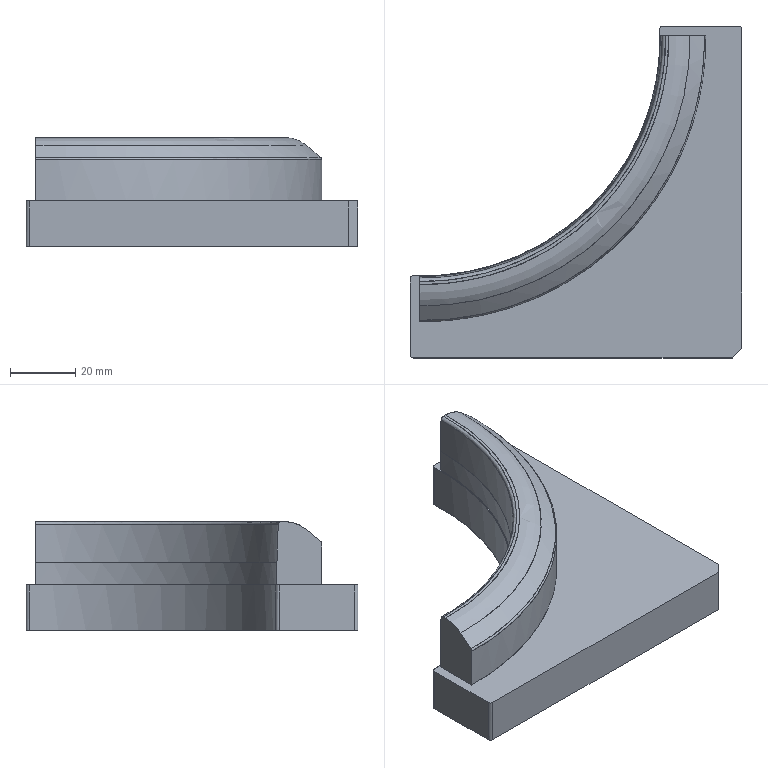NC program | PowerMill | posted with a generic post | part box 102 x 102 x 33.478 mm
Lines 26146 to 27280 of 205885:
N26243 M6
N26244 S8500 M03
N26245 G00 G90 X0.0 Y0.0
N26246 G43 Z11.798 H3
N26247
N26248 G05 P10000 R8
N26249 X37.5844 Y54.0857
N26250 Z0.7984
N26251 G01 Z-0.4016 F360.0
N26252 X33.1677 Y51.2016 F600.0
N26253 X22.0307 Y45.7859
N26254 X21.9859 Y44.2514
N26255 X21.9868 Y43.8083
N26256 X21.9186 Y42.9165
N26257 X21.8632 Y42.0238
N26258 X21.7548 Y40.6849
N26259 X21.6903 Y40.061
N26260 X34.2629 Y46.1749
N26261 X34.2244 Y44.6963
N26262 X34.2103 Y43.798
N26263 X34.1806 Y43.3523
N26264 X34.1258 Y42.0078
N26265 X33.9991 Y40.4872
N26266 X20.8197 Y34.0783
N26267 X20.719 Y33.5435
N26268 X20.4371 Y32.2041
N26269 X20.2385 Y31.3119
N26270 X19.7939 Y29.5261
N26271 X19.555 Y28.6339
N26272 X19.3094 Y27.7845
N26273 X33.3175 Y34.5964
N26274 X33.2791 Y34.4009
N26275 X33.2129 Y33.9562
N26276 X33.0631 Y33.0592
N26277 X32.8983 Y32.1648
N26278 X32.8079 Y31.717
N26279 X32.728 Y31.2672
N26280 X32.6288 Y30.8219
N26281 X32.4611 Y29.9296
N26282 X32.3634 Y29.4765
N26283 X32.2815 Y29.1526
N26284 X32.2658 Y29.0289
N26285 X32.1192 Y28.4543
N26286 X16.9967 Y21.1005
N26287 X16.8928 Y20.8373
N26288 X16.4531 Y19.7915
N26289 X16.0002 Y18.7513
N26290 X15.5539 Y17.7745
N26291 X15.1078 Y16.842
N26292 X14.3017 Y15.2433
N26293 X13.5777 Y13.8786
N26294 X30.3315 Y22.0256
N26295 X29.9768 Y20.977
N26296 X29.8344 Y20.5279
N26297 X29.5964 Y19.8574
N26298 X29.5319 Y19.6308
N26299 X29.3568 Y19.1846
N26300 X28.517 Y16.9457
N26301 X28.2532 Y16.3376
N26302 X28.1539 Y16.058
N26303 X27.799 Y15.2347
N26304 X8.4035 Y5.803
N26305 X7.438 Y4.5314
N26306 X6.6273 Y3.5171
N26307 X5.6141 Y2.2997
N26308 X4.4534 Y0.9605
N26309 X3.6379 Y0.0682
N26310 X2.3615 Y-1.271
N26311 X1.2711 Y-2.3584
N26312 X0.0766 Y-3.5028
N26313 X-0.6368 Y-4.1524
N26314 X24.2797 Y7.964
N26315 X23.6272 Y6.8079
N26316 X23.0209 Y5.7571
N26317 X22.8817 Y5.5385
N26318 X22.4904 Y4.8665
N26319 X22.2152 Y4.4146
N26320 X21.9894 Y4.074
N26321 X21.9399 Y3.9724
N26322 X21.6728 Y3.5169
N26323 X21.5376 Y3.3319
N26324 X20.496 Y1.7334
N26325 X19.8738 Y0.8394
N26326 X19.747 Y0.6317
N26327 X19.5617 Y0.3879
N26328 X19.2643 Y-0.0342
N26329 X-50.1432 Y-33.7859
N26330 X-50.5619 Y-33.584
N26331 X-51.0189 Y-33.3011
N26332 X-51.1992 Y-33.1566
N26333 X-51.4726 Y-32.9584
N26334 X-51.9281 Y-32.5206
N26335 X-52.3807 Y-31.9598
N26336 X-52.4955 Y-31.7858
N26337 X-52.7543 Y-31.335
N26338 X-52.8365 Y-31.1755
N26339 X-52.9621 Y-30.875
N26340 X-53.121 Y-30.4198
N26341 X-53.2371 Y-29.9645
N26342 X-53.2731 Y-29.7486
N26343 X-35.3955 Y-21.055
N26344 X-36.2214 Y-21.1929
N26345 X-37.5607 Y-21.3923
N26346 X-38.453 Y-21.5093
N26347 X-39.7921 Y-21.6633
N26348 X-41.2767 Y-21.8027
N26349 X-42.0235 Y-21.8609
N26350 X-44.256 Y-21.9953
N26351 X-45.5942 Y-22.0335
N26352 X-48.283 Y-22.0454
N26353 X-48.7396 Y-22.0849
N26354 X-49.0718 Y-22.1462
N26355 X-51.4722 Y-23.3135
N26356 X-51.8063 Y-23.6241
N26357 X-52.2062 Y-24.0775
N26358 X-52.3813 Y-24.3133
N26359 X-52.5246 Y-24.5356
N26360 X-52.8361 Y-25.0973
N26361 X-52.9864 Y-25.4462
N26362 X-53.1396 Y-25.9015
N26363 X-53.2501 Y-26.3572
N26364 X-53.3185 Y-26.8125
N26365 X-53.3483 Y-27.2595
N26366 X-53.3469 Y-29.0617
N26367 X-53.3117 Y-29.5175
N26368 X-53.2353 Y-29.9728
N26369 X-53.1185 Y-30.4281
N26370 X-52.96 Y-30.8806
N26371 X-52.8331 Y-31.1829
N26372 X-52.7522 Y-31.3388
N26373 X-52.4922 Y-31.7911
N26374 X-52.3751 Y-31.9675
N26375 X-51.9195 Y-32.5299
N26376 X-51.4618 Y-32.9674
N26377 X-51.1992 Y-33.1566
N26378 X-51.0089 Y-33.3082
N26379 X-50.5527 Y-33.589
N26380 X-50.098 Y-33.8073
N26381 X-49.6389 Y-33.9813
N26382 X-49.2871 Y-34.0663
N26383 X-49.1861 Y-34.1055
N26384 X-48.7298 Y-34.1872
N26385 X-48.2778 Y-34.2252
N26386 X-47.3858 Y-34.2554
N26387 X-46.9306 Y-34.2878
N26388 X-43.3523 Y-34.183
N26389 X-41.3391 Y-34.0705
N26390 X-40.2159 Y-33.9911
N26391 X-39.7718 Y-33.9337
N26392 X-38.8875 Y-33.8718
N26393 X11.5549 Y-9.3425
N26394 G00 Z11.798
N26395 G05 P0
N26396 (---------------)
N26397 ( END TOOLPATH : 粗公基准台01-平坦面平行-D10 )
N26398 (---------------)
N26399 ( START TOOLPATH : 粗公基准台01-基准面偏置-D10 )
N26400 (---------------)
N26401 G00 X0.0 Y0.0 Z9.7984
N26402 G05 P10000 R8
N26403 X-47.0962 Y-15.1649
N26404 Z-18.48
N26405 G01 Z-19.68 F360.0
N26406 X-47.1446 Y-20.4396 F600.0
N26407 X-47.1454 Y-20.8521
N26408 X-46.7492 Y-20.8544
N26409 G03 X-36.4485 Y-20.0287 I-0.2347 J67.5975
N26410 G01 X-35.1254 Y-19.809
N26411 X-34.0714 Y-19.6132
N26412 G03 X-30.902 Y-18.9199 I-14.1754 J72.3923
N26413 G01 X-29.3173 Y-18.5137
N26414 X-27.7326 Y-18.0656
N26415 X-26.1479 Y-17.5743
N26416 G03 X-23.4504 Y-16.6395 I-24.3574 J74.6492
N26417 G03 X-20.6013 Y-15.5106 I-26.3182 J70.5771
N26418 G01 X-19.0166 Y-14.8188
N26419 X-17.4319 Y-14.0768
N26420 X-16.2101 Y-13.4701
N26421 X-14.6989 Y-12.6777
N26422 X-13.4701 Y-11.9945
N26423 X-11.9303 Y-11.093
N26424 X-10.6489 Y-10.3007
N26425 X-9.4309 Y-9.5083
N26426 X-7.9236 Y-8.4761
N26427 G03 X-5.5465 Y-6.7242 I-48.6851 J68.549
N26428 G01 X-4.0663 Y-5.5465
N26429 X-3.1114 Y-4.7542
N26430 X-2.1983 Y-3.9618
N26431 X-1.4913 Y-3.3322
N26432 X-0.7924 Y-2.6936
N26433 G03 X2.6936 Y0.7924 I-48.0043 J51.4903
N26434 G01 X3.3322 Y1.4913
N26435 X3.9618 Y2.1983
N26436 X4.7542 Y3.1114
N26437 X5.5465 Y4.0663
N26438 X6.7242 Y5.5465
N26439 G03 X8.622 Y8.133 I-61.7356 J47.2857
N26440 G01 X9.5083 Y9.4309
N26441 X10.3007 Y10.6489
N26442 X11.093 Y11.9303
N26443 X11.9945 Y13.4701
N26444 X12.6777 Y14.6989
N26445 X13.4701 Y16.2101
N26446 X13.9709 Y17.2187
N26447 G03 X17.3096 Y25.3555 I-60.677 J29.6508
N26448 G01 X17.5743 Y26.1479
N26449 X18.0292 Y27.6134
N26450 X18.5137 Y29.3173
N26451 X18.7179 Y30.1097
N26452 G03 X19.4523 Y33.2791 I-58.6182 J15.251
N26453 G01 X19.6132 Y34.0714
N26454 X19.809 Y35.1254
N26455 G03 X20.8528 Y47.5416 I-66.9151 J11.8775
N26456 G01 X20.8629 Y48.3339
N26457 X20.9029 Y48.7301
N26458 X20.9743 Y49.1263
N26459 X21.0775 Y49.5225
N26460 X21.215 Y49.9186
N26461 X21.3937 Y50.3226
N26462 X21.6065 Y50.711
N26463 X21.8681 Y51.1041
N26464 X22.1861 Y51.4972
N26465 X22.3805 Y51.703
N26466 X22.5853 Y51.8984
N26467 X22.9784 Y52.2199
N26468 X23.4272 Y52.5179
N26469 X23.7708 Y52.7043
N26470 X24.167 Y52.8807
N26471 X24.5631 Y53.02
N26472 X24.8084 Y53.0881
N26473 X25.3555 Y53.1972
N26474 X25.7517 Y53.2383
N26475 X26.1479 Y53.2506
N26476 X40.0141 Y53.2476
N26477 X40.4103 Y53.2188
N26478 X40.7709 Y53.1665
N26479 X41.2027 Y53.0695
N26480 X41.5989 Y52.946
N26481 X41.995 Y52.7863
N26482 X42.3912 Y52.5872
N26483 X42.8555 Y52.2957
N26484 X43.2176 Y52.0173
N26485 X43.5798 Y51.6821
N26486 X43.7477 Y51.5034
N26487 X44.0688 Y51.1072
N26488 X44.3721 Y50.6452
N26489 X44.5653 Y50.2819
N26490 X44.7242 Y49.9186
N26491 X44.8615 Y49.5225
N26492 X44.9648 Y49.1263
N26493 X45.0363 Y48.7301
N26494 X45.077 Y48.3339
N26495 G02 X44.9942 Y42.7874 I-82.7077 J-1.5393
N26496 G01 X44.9556 Y41.995
N26497 X44.8557 Y40.4103
N26498 X44.7629 Y39.2211
N26499 X44.6538 Y38.0332
N26500 X44.4859 Y36.4485
N26501 X44.2893 Y34.8638
N26502 X43.9427 Y32.4867
N26503 X43.5295 Y30.1097
N26504 X43.2207 Y28.5249
N26505 X42.8803 Y26.9402
N26506 X42.6065 Y25.7497
N26507 X42.3162 Y24.5631
N26508 X41.9045 Y22.9784
N26509 G02 X40.9829 Y19.809 I-83.4194 J22.5373
N26510 G01 X40.7376 Y19.0166
N26511 X40.2177 Y17.4319
N26512 X39.618 Y15.7272
N26513 X38.8256 Y13.6071
N26514 X38.0332 Y11.6416
N26515 X37.2409 Y9.7915
N26516 X36.4485 Y8.0489
N26517 X35.6562 Y6.3915
N26518 G02 X31.7176 Y-0.7924 I-84.1319 J41.4541
N26519 G01 X30.902 Y-2.1163
N26520 X30.3081 Y-3.0421
N26521 X29.705 Y-3.9618
N26522 X28.8971 Y-5.1556
N26523 X28.0738 Y-6.3389
N26524 G02 X25.3555 Y-9.9718 I-83.8684 J59.9205
N26525 G01 X24.5838 Y-10.9321
N26526 X23.8033 Y-11.8854
N26527 X22.9784 Y-12.8642
N26528 X22.1912 Y-13.7718
N26529 X21.3937 Y-14.6703
N26530 X20.3127 Y-15.8472
N26531 X19.5615 Y-16.6444
N26532 X18.8 Y-17.4319
N26533 X18.0782 Y-18.1537
N26534 X31.6519 Y-31.7486
N26535 G02 X28.0811 Y-35.1574 I-77.7992 J77.9201
N26536 G01 X27.2583 Y-35.9085
N26537 G03 X27.6697 Y-36.9734 I0.4129 J-0.4524
N26538 G01 X35.5607 Y-36.9919
N26539 G03 X36.8991 Y-35.6541 I0.0032 J1.3352
N26540 G01 X36.8839 Y-27.774
N26541 G03 X35.8188 Y-27.3612 I-0.613 J-0.0011
N26542 G01 X35.0663 Y-28.1831
N26543 G02 X31.6519 Y-31.7486 I-81.2201 J74.3613
N26544 G01 X28.259 Y-28.3504
N26545 G02 X17.1401 Y-38.0098 I-75.0899 J75.2068
N26546 G01 X16.9394 Y-38.1611
N26547 G02 X14.133 Y-40.2033 I-62.0425 J82.3081
N26548 G01 X13.391 Y-40.7244
N26549 G03 X13.7119 Y-41.744 I0.3223 J-0.4589
N26550 G01 X40.3758 Y-41.8091
N26551 G03 X41.7142 Y-40.4713 I0.0033 J1.3351
N26552 G01 X41.6606 Y-13.8346
N26553 G03 X40.6413 Y-13.5124 I-0.5609 J-0.0012
N26554 G01 X40.0065 Y-14.412
N26555 G02 X28.259 Y-28.3504 I-86.8369 J61.268
N26556 G01 X24.8662 Y-24.9523
N26557 G02 X13.5489 Y-34.7012 I-71.7973 J71.9046
N26558 G01 X13.3875 Y-34.8207
N26559 G02 X4.7801 Y-40.5212 I-58.49 J78.9669
N26560 G01 X4.515 Y-40.6775
N26561 G02 X-1.53 Y-43.9616 I-50.2702 J85.3251
N26562 G01 X-2.15 Y-44.2702
N26563 X-4.8771 Y-45.541
N26564 G03 X-4.6651 Y-46.5033 I0.2132 J-0.4575
N26565 G01 X45.1173 Y-46.6262
N26566 G03 X46.0704 Y-46.2294 I0.0033 J1.335
N26567 G01 X46.144 Y-46.1548
N26568 G03 X46.5293 Y-45.2139 I-0.9497 J0.9382
N26569 G01 X46.4279 Y4.4589
N26570 G03 X45.473 Y4.6711 I-0.5013 J-0.001
N26571 G01 X45.0268 Y3.7221
N26572 G02 X24.8662 Y-24.9523 I-91.9576 J43.2299
N26573 G01 X21.4735 Y-21.5543
N26574 G03 X49.8084 Y42.9608 I-68.449 J68.5424
N26575 G01 X49.8203 Y43.2471
N26576 G03 X49.8862 Y47.814 I-84.0295 J3.4964
N26577 G01 X49.8788 Y48.3939
N26578 X49.8658 Y48.6553
N26579 X49.682 Y50.7768
N26580 G02 X50.9206 Y51.0012 I0.6295 J0.0559
N26581 G01 X51.0985 Y50.358
N26582 X51.1281 Y50.2141
N26583 X51.1383 Y50.0675
N26584 X51.3387 Y-47.1476
N26585 G02 X51.2233 Y-47.8213 I-2.0 J-0.0041
N26586 G01 X51.0459 Y-48.3205
N26587 G02 X50.5842 Y-49.0565 I-1.8846 J0.6696
N26588 G01 X49.083 Y-50.5761
N26589 G02 X48.4003 Y-51.0286 I-1.4229 J1.4056
N26590 G01 X47.7332 Y-51.2943
N26591 G02 X46.9882 Y-51.4363 I-0.7401 J1.8581
N26592 G01 X-49.8843 Y-51.1952
N26593 X-50.0249 Y-51.1872
N26594 X-50.1637 Y-51.164
N26595 X-50.947 Y-50.9893
N26596 G02 X-50.7293 Y-49.6728 I0.1455 J0.6522
N26597 G01 X-48.059 Y-49.963
N26598 G03 X-39.4311 Y-49.8087 I3.7057 J34.0962
N26599 G01 X-33.0845 Y-48.8883
N26600 G03 X-4.2777 Y-39.9657 I-13.8969 J95.8287
N26601 G01 X-4.2529 Y-39.9535
N26602 G03 X2.7375 Y-36.1499 I-42.6045 J86.6266
N26603 G01 X3.2663 Y-35.8333
N26604 X4.6777 Y-34.9637
N26605 X5.2385 Y-34.6046
N26606 G03 X8.5517 Y-32.3861 I-53.9623 J84.1743
N26607 G01 X9.106 Y-31.9984
N26608 X9.7715 Y-31.5174
N26609 G03 X21.4735 Y-21.5543 I-56.7471 J78.5057
N26610 G01 X18.0782 Y-18.1537
N26611 X17.4319 Y-18.8
N26612 X16.6444 Y-19.5615
N26613 X15.8472 Y-20.3127
N26614 X14.6703 Y-21.3937
N26615 G02 X9.5083 Y-25.7153 I-62.9677 J69.968
N26616 G02 X6.3389 Y-28.0738 I-61.8179 J79.7641
N26617 G02 X2.1163 Y-30.902 I-58.3984 J82.6239
N26618 G01 X0.7924 Y-31.7176
N26619 G02 X-6.3915 Y-35.6562 I-48.638 J80.1933
N26620 G01 X-8.0489 Y-36.4485
N26621 X-9.171 Y-36.9637
N26622 X-10.3007 Y-37.4622
N26623 X-11.8854 Y-38.1354
N26624 X-13.6071 Y-38.8256
N26625 X-15.7272 Y-39.618
N26626 X-17.4319 Y-40.2177
N26627 X-19.0166 Y-40.7376
N26628 G02 X-22.1861 Y-41.6855 I-31.3609 J99.0877
N26629 G01 X-22.9784 Y-41.9045
N26630 X-24.5631 Y-42.3162
N26631 X-25.7497 Y-42.6065
N26632 X-26.9402 Y-42.8803
N26633 X-28.5249 Y-43.2207
N26634 X-30.5053 Y-43.6037
N26635 X-32.4867 Y-43.9427
N26636 X-34.8638 Y-44.2893
N26637 X-36.4485 Y-44.4859
N26638 X-38.0332 Y-44.6538
N26639 X-39.2211 Y-44.7629
N26640 X-40.4103 Y-44.8557
N26641 X-41.995 Y-44.9556
N26642 G02 X-47.5416 Y-45.0894 I-4.9154 J88.6891
N26643 G01 X-48.3339 Y-45.077
N26644 X-48.7301 Y-45.0366
N26645 X-49.1263 Y-44.9648
N26646 X-49.5225 Y-44.8619
N26647 X-49.9186 Y-44.7242
N26648 X-50.2819 Y-44.5659
N26649 X-50.711 Y-44.3334
N26650 X-51.1072 Y-44.069
N26651 X-51.5034 Y-43.7477
N26652 X-51.6821 Y-43.5798
N26653 X-52.0169 Y-43.2176
N26654 X-52.3429 Y-42.7874
N26655 X-52.587 Y-42.3912
N26656 X-52.7863 Y-41.995
N26657 X-52.9462 Y-41.5989
N26658 X-53.0881 Y-41.1315
N26659 X-53.1668 Y-40.7709
N26660 X-53.2188 Y-40.4103
N26661 X-53.2478 Y-40.0141
N26662 X-53.2506 Y-26.1479
N26663 X-53.2385 Y-25.7517
N26664 X-53.1972 Y-25.3555
N26665 X-53.0881 Y-24.8084
N26666 X-53.02 Y-24.5631
N26667 X-52.8806 Y-24.167
N26668 X-52.7043 Y-23.7708
N26669 X-52.5177 Y-23.4272
N26670 X-52.2957 Y-23.0837
N26671 X-52.2199 Y-22.9784
N26672 X-51.8983 Y-22.5853
N26673 X-51.7032 Y-22.3802
N26674 X-51.4972 Y-22.1861
N26675 X-51.1041 Y-21.8682
N26676 X-50.711 Y-21.6065
N26677 X-50.3226 Y-21.3937
N26678 X-49.9186 Y-21.215
N26679 X-49.5225 Y-21.0776
N26680 X-49.1263 Y-20.9743
N26681 X-48.7301 Y-20.903
N26682 X-48.3339 Y-20.8629
N26683 X-47.1454 Y-20.8521
N26684 X-47.1446 Y-20.4396
N26685 G00 Z9.7984
N26686 G05 P0
N26687 (---------------)
N26688 ( END TOOLPATH : 粗公基准台01-基准面偏置-D10 )
N26689 (---------------)
N26690 ( START TOOLPATH : 粗公基准台01-外形侧光-D10 )
N26691 (---------------)
N26692 G00 X0.0 Y0.0 Z10.798
N26693 G05 P10000 R8
N26694 X18.943 Y-17.3914
N26695 Z-14.65
N26696 G01 Z-19.65 F360.0
N26697 G03 X17.8825 Y-17.8311 I0.0006 J-1.5 F600.0
N26698 G02 X12.8329 Y-22.5204 I-65.2186 J65.1672
N26699 G01 X11.4091 Y-23.7209
N26700 G02 X9.8587 Y-24.9733 I-114.9081 J140.6612
N26701 G01 X8.3089 Y-26.171
N26702 G02 X-8.4201 Y-36.2142 I-55.4787 J73.4569
N26703 G02 X-26.8308 Y-42.4776 I-38.6173 J83.3227
N26704 G02 X-28.6393 Y-42.8661 I-49.578 J226.3665
N26705 G02 X-48.0187 Y-44.717 I-18.3715 J89.9759
N26706 G02 X-52.88 Y-39.7554 I0.0201 J4.882
N26707 G01 X-52.8799 Y-26.0707
N26708 G02 X-48.0161 Y-21.2224 I4.88 J-0.0317
N26709 G03 X-21.7145 Y-16.3702 I0.9854 J68.3689
N26710 G03 X16.3702 Y21.7145 I-25.299 J63.3837
N26711 G03 X21.2225 Y48.0187 I-63.5212 J25.3172
N26712 G02 X26.0734 Y52.8799 I4.88 J-0.0188
N26713 G01 X37.1545 Y52.88
N26714 X39.7564
N26715 G02 X44.717 Y48.0166 I0.0786 J-4.8814
N26716 G02 X42.8658 Y28.6381 I-91.9079 J-0.9979
N26717 G01 X42.4773 Y26.8296
N26718 G02 X36.2137 Y8.419 I-89.8562 J20.2997
N26719 G02 X24.9723 Y-9.86 I-83.4077 J38.6988
N26720 G02 X22.5196 Y-12.8338 I-74.6487 J59.0703
N26721 G02 X17.8825 Y-17.8311 I-69.8563 J60.1705
N26722 G03 X17.4436 Y-18.892 I1.061 J-1.0603
N26723 G01 X18.8864 Y-17.3348
N26724 G03 X17.8259 Y-17.7746 I0.0006 J-1.5
N26725 G02 X12.7813 Y-22.4592 I-65.1634 J65.1122
N26726 G01 X11.3587 Y-23.6588
N26727 G02 X9.8098 Y-24.91 I-115.0842 J140.8779
N26728 G01 X8.2609 Y-26.1071
N26729 G02 X-8.453 Y-36.1413 I-55.4308 J73.3931
N26730 G02 X-26.8478 Y-42.3994 I-38.5844 J83.2499
N26731 G02 X-28.6549 Y-42.7876 I-49.6123 J226.5227
N26732 G02 X-48.0163 Y-44.637 I-18.3562 J89.8994
N26733 G02 X-52.8 Y-39.7554 I0.0177 J4.802
N26734 G01 X-52.7999 Y-26.0734
N26735 G02 X-48.0163 Y-21.3024 I4.7999 J-0.029
N26736 G03 X-21.6848 Y-16.4445 I0.9857 J68.4487
N26737 G03 X16.4445 Y21.6848 I-25.3287 J63.458
N26738 G03 X21.3024 Y48.0163 I-63.5914 J25.3459
N26739 G02 X26.0734 Y52.7999 I4.8 J-0.0163
N26740 G01 X37.1545 Y52.8
N26741 X39.7554
N26742 G02 X44.637 Y48.0163 I0.0796 J-4.8014
N26743 G02 X42.7876 Y28.6549 I-91.8291 J-0.9974
N26744 G01 X42.3994 Y26.8478
N26745 G02 X36.1413 Y8.453 I-89.7783 J20.2815
N26746 G02 X24.91 Y-9.8098 I-83.3356 J38.665
N26747 G02 X22.4592 Y-12.7813 I-74.5881 J59.0216
N26748 G02 X17.8259 Y-17.7746 I-69.7956 J60.1177
N26749 G03 X17.387 Y-18.8354 I1.0611 J-1.0602
N26750 G00 Z10.798
N26751 G05 P0
N26752 (---------------)
N26753 ( END TOOLPATH : 粗公基准台01-外形侧光-D10 )
N26754 (---------------)
N26755 ( START TOOLPATH : 粗公基准台01-基准台侧光-D10 )
N26756 (---------------)
N26757 G00 X0.0 Y0.0 Z9.7984
N26758 G05 P10000 R8
N26759 X55.9652 Y-57.2901
N26760 Z-32.38
N26761 G01 Z-33.58 F360.0
N26762 G03 X52.4296 Y-53.7546 I-1.7678 J1.7677 F600.0
N26763 G01 X51.6834 Y-54.5008
N26764 X51.6828 Y-54.5015
N26765 X51.6821 Y-54.5021
N26766 X51.3559 Y-54.8136
N26767 X51.3542 Y-54.8151
N26768 X51.3525 Y-54.8167
N26769 X51.2317 Y-54.9195
N26770 X51.2295 Y-54.9213
N26771 X51.2272 Y-54.9231
N26772 X50.7802 Y-55.2516
N26773 X50.7767 Y-55.254
N26774 X50.7731 Y-55.2563
N26775 X50.3261 Y-55.516
N26776 X50.3225 Y-55.518
N26777 X50.3189 Y-55.5197
N26778 X49.8716 Y-55.7226
N26779 X49.868 Y-55.7241
N26780 X49.8644 Y-55.7254
N26781 X49.4178 Y-55.8781
N26782 X49.4142 Y-55.8792
N26783 X49.4106 Y-55.8801
N26784 X48.9636 Y-55.9877
N26785 X48.9601 Y-55.9885
N26786 X48.9565 Y-55.9891
N26787 X48.5095 Y-56.0543
N26788 X48.5059 Y-56.0547
N26789 X48.5023 Y-56.055
N26790 X48.0554 Y-56.0796
N26791 X48.0532 Y-56.0797
N26792 X48.051 Y-56.0798
N26793 X-49.8389 Y-56.08
N26794 X-49.8396
N26795 X-49.8404
N26796 X-50.2873 Y-56.0718
N26797 X-50.2899 Y-56.0717
N26798 X-50.2925 Y-56.0716
N26799 X-50.7395 Y-56.0345
N26800 X-50.7425 Y-56.0342
N26801 X-50.7456 Y-56.0338
N26802 X-51.1926 Y-55.9619
N26803 X-51.1956 Y-55.9613
N26804 X-51.1986 Y-55.9606
N26805 X-51.6456 Y-55.8527
N26806 X-51.6485 Y-55.8519
N26807 X-51.6513 Y-55.8511
N26808 X-52.041 Y-55.7259
N26809 X-52.0439 Y-55.7249
N26810 X-52.0467 Y-55.7238
N26811 X-52.551 Y-55.5185
N26812 X-52.5544 Y-55.517
N26813 X-52.5577 Y-55.5154
N26814 X-53.0047 Y-55.2831
N26815 X-53.0074 Y-55.2816
N26816 X-53.0101 Y-55.28
N26817 X-53.4571 Y-55.0012
N26818 X-53.4596 Y-54.9996
N26819 X-53.4621 Y-54.9979
N26820 X-53.7044 Y-54.8203
N26821 X-53.7061 Y-54.8189
N26822 X-53.7079 Y-54.8176
N26823 X-53.9125 Y-54.6494
N26824 X-53.9138 Y-54.6484
N26825 X-53.9149 Y-54.6474
N26826 X-54.2285 Y-54.3685
N26827 X-54.2302 Y-54.367
N26828 X-54.2318 Y-54.3653
N26829 X-54.3653 Y-54.2318
N26830 X-54.367 Y-54.2302
N26831 X-54.3685 Y-54.2285
N26832 X-54.6474 Y-53.9149
N26833 X-54.6484 Y-53.9138
N26834 X-54.6494 Y-53.9125
N26835 X-54.8176 Y-53.7079
N26836 X-54.8189 Y-53.7061
N26837 X-54.8203 Y-53.7044
N26838 X-54.9979 Y-53.4621
N26839 X-54.9996 Y-53.4596
N26840 X-55.0012 Y-53.4571
N26841 X-55.28 Y-53.0101
N26842 X-55.2816 Y-53.0074
N26843 X-55.2831 Y-53.0047
N26844 X-55.5154 Y-52.5577
N26845 X-55.5169 Y-52.5546
N26846 X-55.5183 Y-52.5514
N26847 X-55.7032 Y-52.1044
N26848 X-55.7043 Y-52.1015
N26849 X-55.7053 Y-52.0986
N26850 X-55.851 Y-51.6516
N26851 X-55.8519 Y-51.6486
N26852 X-55.8527 Y-51.6456
N26853 X-55.9606 Y-51.1986
N26854 X-55.9613 Y-51.1956
N26855 X-55.9619 Y-51.1926
N26856 X-56.0338 Y-50.7456
N26857 X-56.0342 Y-50.7425
N26858 X-56.0345 Y-50.7395
N26859 X-56.0716 Y-50.2925
N26860 X-56.0717 Y-50.2899
N26861 X-56.0718 Y-50.2873
N26862 X-56.08 Y-49.8404
N26863 Y-49.8396
N26864 Y-49.8389
N26865 Y-27.0426
N26866 Y-27.0425
N26867 Y-27.0423
N26868 X-56.078 Y-26.5953
N26869 Y-26.5929
N26870 X-56.0779 Y-26.5905
N26871 X-56.0488 Y-26.1435
N26872 X-56.0486 Y-26.1408
N26873 X-56.0483 Y-26.1382
N26874 X-55.9895 Y-25.6912
N26875 X-55.989 Y-25.6878
N26876 X-55.9883 Y-25.6844
N26877 X-55.8893 Y-25.2374
N26878 X-55.8887 Y-25.2349
N26879 X-55.888 Y-25.2324
N26880 X-55.7585 Y-24.7854
N26881 X-55.7574 Y-24.7821
N26882 X-55.7562 Y-24.7788
N26883 X-55.5828 Y-24.3318
N26884 X-55.5816 Y-24.329
N26885 X-55.5804 Y-24.3262
N26886 X-55.3669 Y-23.8793
N26887 X-55.3658 Y-23.8771
N26888 X-55.3647 Y-23.8749
N26889 X-55.2727 Y-23.7091
N26890 X-55.2718 Y-23.7075
N26891 X-55.2709 Y-23.706
N26892 X-55.0981 Y-23.4249
N26893 X-55.0967 Y-23.4227
N26894 X-55.0953 Y-23.4206
N26895 X-54.8211 Y-23.0318
N26896 X-54.8187 Y-23.0286
N26897 X-54.8162 Y-23.0256
N26898 X-54.3692 Y-22.5094
N26899 X-54.3664 Y-22.5063
N26900 X-54.3633 Y-22.5033
N26901 X-53.9164 Y-22.0861
N26902 X-53.9134 Y-22.0835
N26903 X-53.9104 Y-22.081
N26904 X-53.4634 Y-21.7391
N26905 X-53.4604 Y-21.737
N26906 X-53.4573 Y-21.7349
N26907 X-53.0104 Y-21.4541
N26908 X-53.0074 Y-21.4523
N26909 X-53.0045 Y-21.4507
N26910 X-52.5575 Y-21.2203
N26911 X-52.5544 Y-21.2188
N26912 X-52.5514 Y-21.2175
N26913 X-52.1044 Y-21.0328
N26914 X-52.1015 Y-21.0317
N26915 X-52.0986 Y-21.0307
N26916 X-51.6516 Y-20.8849
N26917 X-51.6485 Y-20.8839
N26918 X-51.6452 Y-20.8831
N26919 X-51.1982 Y-20.7776
N26920 X-51.1957 Y-20.7771
N26921 X-51.1932 Y-20.7766
N26922 X-50.7756 Y-20.706
N26923 X-50.7722 Y-20.7055
N26924 X-50.7688 Y-20.7051
N26925 X-50.2924 Y-20.6662
N26926 X-50.2898 Y-20.666
N26927 X-50.2872 Y-20.6659
N26928 X-49.8402 Y-20.6584
N26929 X-49.8384
N26930 X-49.8366
N26931 X-48.4964 Y-20.6973
N26932 X-46.7102 Y-20.7136
N26933 X-45.3711 Y-20.6941
N26934 X-43.5851 Y-20.6276
N26935 X-41.7991 Y-20.5159
N26936 X-40.4601 Y-20.3987
N26937 X-38.674 Y-20.2005
N26938 X-37.3349 Y-20.0211
N26939 X-35.5488 Y-19.7382
N26940 X-34.2096 Y-19.4945
N26941 X-32.4235 Y-19.128
N26942 X-31.0843 Y-18.8184
N26943 X-29.745 Y-18.4788
N26944 X-28.1068 Y-18.0261
N26945 X-26.6356 Y-17.5797
N26946 X-24.8338 Y-16.9826
N26947 X-23.4945 Y-16.5029
N26948 X-22.1552 Y-15.9911
N26949 X-20.5764 Y-15.3473
N26950 X-19.0299 Y-14.6689
N26951 X-17.6906 Y-14.043
N26952 X-16.3512 Y-13.3809
N26953 X-15.0118 Y-12.6816
N26954 X-13.6724 Y-11.9438
N26955 X-12.3331 Y-11.1664
N26956 X-10.9937 Y-10.3477
N26957 X-9.6543 Y-9.485
N26958 X-8.315 Y-8.5767
N26959 X-6.9756 Y-7.6191
N26960 X-5.6362 Y-6.6111
N26961 X-4.2967 Y-5.5519
N26962 X-3.1884 Y-4.6323
N26963 X-2.0646 Y-3.6578
N26964 X-0.6878 Y-2.3999
N26965 X0.1678 Y-1.5844
N26966 X0.614 Y-1.1455
N26967 X1.5845 Y-0.1677
N26968 X2.3999 Y0.6878
N26969 X3.6579 Y2.0647
N26970 X4.4339 Y2.9573
N26971 X5.5252 Y4.2635
N26972 X6.6111 Y5.6362
N26973 X7.619 Y6.9756
N26974 X8.5767 Y8.315
N26975 X9.485 Y9.6543
N26976 X10.3477 Y10.9937
N26977 X11.1664 Y12.3331
N26978 X11.9439 Y13.6724
N26979 X12.6816 Y15.0118
N26980 X13.3809 Y16.3512
N26981 X14.043 Y17.6906
N26982 X14.6689 Y19.0299
N26983 X15.3473 Y20.5764
N26984 X15.9911 Y22.1552
N26985 X16.5029 Y23.4945
N26986 X16.9826 Y24.8338
N26987 X17.5797 Y26.6356
N26988 X18.0261 Y28.107
N26989 X18.3598 Y29.2983
N26990 X18.8185 Y31.0845
N26991 X19.128 Y32.4236
N26992 X19.4074 Y33.7629
N26993 X19.7382 Y35.5489
N26994 X20.021 Y37.3349
N26995 X20.2005 Y38.674
N26996 X20.3987 Y40.4601
N26997 X20.5159 Y41.7993
N26998 X20.6037 Y43.1385
N26999 X20.6819 Y44.9245
N27000 X20.7136 Y46.7105
N27001 X20.7047 Y48.1703
N27002 X20.6584 Y49.8367
N27003 Y49.8385
N27004 Y49.8402
N27005 X20.6659 Y50.2872
N27006 X20.666 Y50.2897
N27007 X20.6661 Y50.2922
N27008 X20.7013 Y50.7391
N27009 X20.7016 Y50.7426
N27010 X20.7021 Y50.746
N27011 X20.7766 Y51.193
N27012 X20.7771 Y51.1956
N27013 X20.7776 Y51.1982
N27014 X20.8831 Y51.6452
N27015 X20.8839 Y51.6484
N27016 X20.8849 Y51.6516
N27017 X21.0307 Y52.0986
N27018 X21.0317 Y52.1015
N27019 X21.0328 Y52.1044
N27020 X21.2175 Y52.5514
N27021 X21.2189 Y52.5544
N27022 X21.2203 Y52.5575
N27023 X21.4507 Y53.0045
N27024 X21.4523 Y53.0074
N27025 X21.4541 Y53.0104
N27026 X21.7349 Y53.4573
N27027 X21.7369 Y53.4603
N27028 X21.739 Y53.4632
N27029 X22.0621 Y53.888
N27030 X22.0646 Y53.8911
N27031 X22.0672 Y53.894
N27032 X22.5032 Y54.3632
N27033 X22.5061 Y54.3661
N27034 X22.5091 Y54.3689
N27035 X22.967 Y54.7703
N27036 X22.9701 Y54.7728
N27037 X22.9732 Y54.7752
N27038 X23.4202 Y55.095
N27039 X23.4225 Y55.0966
N27040 X23.4249 Y55.0981
N27041 X23.706 Y55.2709
N27042 X23.7075 Y55.2718
N27043 X23.7091 Y55.2727
N27044 X23.8749 Y55.3647
N27045 X23.8771 Y55.3658
N27046 X23.8793 Y55.3669
N27047 X24.3262 Y55.5804
N27048 X24.3287 Y55.5815
N27049 X24.3311 Y55.5825
N27050 X24.6869 Y55.724
N27051 X24.6901 Y55.7253
N27052 X24.6935 Y55.7263
N27053 X25.2317 Y55.8878
N27054 X25.2345 Y55.8886
N27055 X25.2374 Y55.8893
N27056 X25.6844 Y55.9883
N27057 X25.6878 Y55.9889
N27058 X25.6912 Y55.9895
N27059 X26.1382 Y56.0483
N27060 X26.1408 Y56.0485
N27061 X26.1435 Y56.0488
N27062 X26.5904 Y56.0779
N27063 X26.5929 Y56.078
N27064 X26.5953
N27065 X27.0423 Y56.08
N27066 X27.0425
N27067 X27.0426
N27068 X49.8389
N27069 X49.8396
N27070 X49.8404
N27071 X50.2873 Y56.0718
N27072 X50.2899 Y56.0717
N27073 X50.2925 Y56.0716
N27074 X50.7395 Y56.0345
N27075 X50.7425 Y56.0342
N27076 X50.7456 Y56.0338
N27077 X51.1926 Y55.9619
N27078 X51.1956 Y55.9613
N27079 X51.1986 Y55.9606
N27080 X51.6456 Y55.8527
N27081 X51.6485 Y55.8519
N27082 X51.6513 Y55.8511
N27083 X52.041 Y55.7259
N27084 X52.0439 Y55.7249
N27085 X52.0467 Y55.7238
N27086 X52.551 Y55.5185
N27087 X52.5544 Y55.517
N27088 X52.5577 Y55.5154
N27089 X53.0047 Y55.2831
N27090 X53.0074 Y55.2816
N27091 X53.0101 Y55.28
N27092 X53.4571 Y55.0012
N27093 X53.4596 Y54.9996
N27094 X53.4621 Y54.9979
N27095 X53.7044 Y54.8203
N27096 X53.7061 Y54.8189
N27097 X53.7079 Y54.8176
N27098 X53.9125 Y54.6494
N27099 X53.9138 Y54.6484
N27100 X53.9149 Y54.6474
N27101 X54.2285 Y54.3685
N27102 X54.2302 Y54.367
N27103 X54.2318 Y54.3653
N27104 X54.3653 Y54.2318
N27105 X54.367 Y54.2302
N27106 X54.3685 Y54.2285
N27107 X54.6474 Y53.9149
N27108 X54.6484 Y53.9138
N27109 X54.6494 Y53.9125
N27110 X54.8176 Y53.7079
N27111 X54.8189 Y53.7061
N27112 X54.8203 Y53.7044
N27113 X54.9979 Y53.4621
N27114 X54.9996 Y53.4596
N27115 X55.0012 Y53.4571
N27116 X55.28 Y53.0101
N27117 X55.2816 Y53.0074
N27118 X55.2831 Y53.0047
N27119 X55.5154 Y52.5577
N27120 X55.517 Y52.5546
N27121 X55.5184 Y52.5514
N27122 X55.7032 Y52.1044
N27123 X55.7043 Y52.1015
N27124 X55.7053 Y52.0986
N27125 X55.851 Y51.6516
N27126 X55.8519 Y51.6486
N27127 X55.8527 Y51.6456
N27128 X55.9606 Y51.1986
N27129 X55.9613 Y51.1956
N27130 X55.9618 Y51.1926
N27131 X56.0338 Y50.7456
N27132 X56.0342 Y50.7425
N27133 X56.0345 Y50.7395
N27134 X56.0715 Y50.2925
N27135 X56.0717 Y50.2899
N27136 X56.0718 Y50.2874
N27137 X56.08 Y49.8404
N27138 Y49.8396
N27139 Y49.8389
N27140 X56.0799 Y0.894
N27141 X56.0798 Y-48.051
N27142 X56.0797 Y-48.0532
N27143 X56.0796 Y-48.0554
N27144 X56.055 Y-48.5023
N27145 X56.0547 Y-48.5059
N27146 X56.0543 Y-48.5095
N27147 X55.9891 Y-48.9565
N27148 X55.9885 Y-48.9601
N27149 X55.9877 Y-48.9636
N27150 X55.8801 Y-49.4106
N27151 X55.8792 Y-49.4142
N27152 X55.8781 Y-49.4178
N27153 X55.7254 Y-49.8644
N27154 X55.7241 Y-49.868
N27155 X55.7226 Y-49.8716
N27156 X55.5197 Y-50.3189
N27157 X55.518 Y-50.3224
N27158 X55.5162 Y-50.3259
N27159 X55.272 Y-50.7487
N27160 X55.2698 Y-50.7524
N27161 X55.2673 Y-50.7559
N27162 X54.9232 Y-51.227
N27163 X54.9214 Y-51.2294
N27164 X54.9195 Y-51.2317
N27165 X54.8167 Y-51.3525
N27166 X54.8151 Y-51.3542
N27167 X54.8136 Y-51.3559
N27168 X54.5021 Y-51.6821
N27169 X54.5015 Y-51.6828
N27170 X54.5008 Y-51.6834
N27171 X52.4296 Y-53.7546
N27172 G03 X55.9652 Y-57.2901 I1.7678 J-1.7678
N27173 G01 X55.9137 Y-57.2285
N27174 G03 X52.3781 Y-53.693 I-1.7678 J1.7678
N27175 G01 X51.6268 Y-54.4442
N27176 X51.3007 Y-54.7557
N27177 X51.1799 Y-54.8586
N27178 X50.7329 Y-55.1871
N27179 X50.2859 Y-55.4469
N27180 X49.8386 Y-55.6497
N27181 X49.3919 Y-55.8024
N27182 X48.9449 Y-55.9099
N27183 X48.4979 Y-55.9751
N27184 X48.051 Y-55.9998
N27185 X-49.8389 Y-56.0
N27186 X-50.2859 Y-55.9918
N27187 X-50.7329 Y-55.9548
N27188 X-51.1799 Y-55.8829
N27189 X-51.6268 Y-55.7749
N27190 X-52.0166 Y-55.6497
N27191 X-52.5208 Y-55.4444
N27192 X-52.9678 Y-55.2121
N27193 X-53.4148 Y-54.9333
N27194 X-53.6571 Y-54.7557
N27195 X-53.8618 Y-54.5876
N27196 X-54.1753 Y-54.3088
N27197 X-54.3088 Y-54.1753
N27198 X-54.5876 Y-53.8618
N27199 X-54.7557 Y-53.6571
N27200 X-54.9333 Y-53.4148
N27201 X-55.2121 Y-52.9678
N27202 X-55.4444 Y-52.5208
N27203 X-55.6292 Y-52.0738
N27204 X-55.7749 Y-51.6268
N27205 X-55.8829 Y-51.1799
N27206 X-55.9548 Y-50.7329
N27207 X-55.9918 Y-50.2859
N27208 X-56.0 Y-49.8389
N27209 Y-27.0426
N27210 X-55.998 Y-26.5956
N27211 X-55.969 Y-26.1487
N27212 X-55.9102 Y-25.7017
N27213 X-55.8112 Y-25.2547
N27214 X-55.6816 Y-24.8077
N27215 X-55.5082 Y-24.3607
N27216 X-55.2947 Y-23.9137
N27217 X-55.2027 Y-23.7479
N27218 X-55.0299 Y-23.4667
N27219 X-54.7557 Y-23.0779
N27220 X-54.3088 Y-22.5618
N27221 X-53.8618 Y-22.1446
N27222 X-53.4148 Y-21.8027
N27223 X-52.9678 Y-21.5218
N27224 X-52.5208 Y-21.2914
N27225 X-52.0738 Y-21.1067
N27226 X-51.6268 Y-20.9609
N27227 X-51.1799 Y-20.8555
N27228 X-50.7623 Y-20.7848
N27229 X-50.2859 Y-20.7459
N27230 X-49.8389 Y-20.7384
N27231 X-48.4979 Y-20.7773
N27232 X-46.71 Y-20.7936
N27233 X-45.369 Y-20.7741
N27234 X-43.5811 Y-20.7075
N27235 X-41.7932 Y-20.5957
N27236 X-40.4522 Y-20.4783
N27237 X-38.6643 Y-20.2799
N27238 X-37.3233 Y-20.1002
N27239 X-35.5354 Y-19.8171
N27240 X-34.1944 Y-19.573
N27241 X-32.4065 Y-19.2061
N27242 X-31.0655 Y-18.8962
N27243 X-29.7245 Y-18.5561
N27244 X-28.0846 Y-18.1029
N27245 X-26.6114 Y-17.6559
N27246 X-24.8077 Y-17.0582
N27247 X-23.4667 Y-16.5779
N27248 X-22.1258 Y-16.0655
N27249 X-20.5452 Y-15.421
N27250 X-18.9969 Y-14.7418
N27251 X-17.6559 Y-14.1151
N27252 X-16.315 Y-13.4522
N27253 X-14.974 Y-12.7521
N27254 X-13.6331 Y-12.0135
N27255 X-12.2921 Y-11.2351
N27256 X-10.9511 Y-10.4155
N27257 X-9.6102 Y-9.5517
N27258 X-8.2692 Y-8.6424
N27259 X-6.9283 Y-7.6836
N27260 X-5.5873 Y-6.6745
N27261 X-4.2464 Y-5.6141
N27262 X-3.1366 Y-4.6933
N27263 X-2.0114 Y-3.7176
N27264 X-0.6333 Y-2.4584
N27265 X0.2235 Y-1.6419
N27266 X0.6705 Y-1.2022
N27267 X1.6419 Y-0.2235
N27268 X2.4584 Y0.6333
N27269 X3.7176 Y2.0114
N27270 X4.4948 Y2.9054
N27271 X5.5873 Y4.213
N27272 X6.6745 Y5.5873
N27273 X7.6835 Y6.9283
N27274 X8.6424 Y8.2692
N27275 X9.5517 Y9.6102
N27276 X10.4154 Y10.9511
N27277 X11.2351 Y12.2921
N27278 X12.0135 Y13.6331
N27279 X12.7521 Y14.974
N27280 X13.4522 Y16.315
N27281 X14.1151 Y17.6559
N27282 X14.7418 Y18.9969
N27283 X15.421 Y20.5452
N27284 X16.0655 Y22.1258
N27285 X16.5779 Y23.4667
N27286 X17.0583 Y24.8077
N27287 X17.6559 Y26.6114
N27288 X18.1029 Y28.0845
N27289 X18.4371 Y29.2776
N27290 X18.8962 Y31.0655
N27291 X19.2061 Y32.4065
N27292 X19.4859 Y33.7474
N27293 X19.817 Y35.5354
N27294 X20.1002 Y37.3233
N27295 X20.2799 Y38.6643
N27296 X20.4783 Y40.4522
N27297 X20.5957 Y41.7932
N27298 X20.6835 Y43.1341
N27299 X20.7619 Y44.9221
N27300 X20.7936 Y46.71
N27301 X20.7848 Y48.1663
N27302 X20.7847 Y48.1717
N27303 X20.7384 Y49.8389
N27304 X20.7459 Y50.2859
N27305 X20.7811 Y50.7329
N27306 X20.8555 Y51.1799
N27307 X20.9609 Y51.6268
N27308 X21.1067 Y52.0738
N27309 X21.2914 Y52.5208
N27310 X21.5218 Y52.9678
N27311 X21.8027 Y53.4148
N27312 X22.1258 Y53.8396
N27313 X22.5618 Y54.3088
N27314 X23.0198 Y54.7101
N27315 X23.4667 Y55.0299
N27316 X23.7479 Y55.2027
N27317 X23.9137 Y55.2947
N27318 X24.3607 Y55.5082
N27319 X24.7165 Y55.6497
N27320 X25.2547 Y55.8112
N27321 X25.7017 Y55.9102
N27322 X26.1487 Y55.9689
N27323 X26.5956 Y55.998
N27324 X27.0426 Y56.0
N27325 X49.8389
N27326 X50.2859 Y55.9918
N27327 X50.7329 Y55.9548
N27328 X51.1799 Y55.8829
N27329 X51.6268 Y55.7749
N27330 X52.0166 Y55.6497
N27331 X52.5208 Y55.4444
N27332 X52.9678 Y55.2121
N27333 X53.4148 Y54.9333
N27334 X53.6571 Y54.7557
N27335 X53.8618 Y54.5876
N27336 X54.1753 Y54.3088
N27337 X54.3088 Y54.1753
N27338 X54.5876 Y53.8618
N27339 X54.7557 Y53.6571
N27340 X54.9333 Y53.4148
N27341 X55.2121 Y52.9678
N27342 X55.4444 Y52.5208
N27343 X55.6292 Y52.0738
N27344 X55.7749 Y51.6268
N27345 X55.8829 Y51.1799
N27346 X55.9548 Y50.7329
N27347 X55.9918 Y50.2859
N27348 X56.0 Y49.8389
N27349 X55.9999 Y0.894
N27350 X55.9998 Y-48.051
N27351 X55.9751 Y-48.4979
N27352 X55.9099 Y-48.9449
N27353 X55.8024 Y-49.3919
N27354 X55.6497 Y-49.8386
N27355 X55.4469 Y-50.2859
N27356 X55.2027 Y-50.7087
N27357 X54.8586 Y-51.1799
N27358 X54.7557 Y-51.3007
N27359 X54.4442 Y-51.6268
N27360 X52.3781 Y-53.693
N27361 G03 X55.9137 Y-57.2285 I1.7678 J-1.7677
N27362 G00 Z9.7984
N27363 G05 P0
N27364 (---------------)
N27365 ( END TOOLPATH : 粗公基准台01-基准台侧光-D10 )
N27366 (---------------)
N27367
N27368 M05
N27369 G53 Z0.0
N27370 (---------------)
N27371 ( START TOOLPATH : 粗公精光01-平行-R2 )
N27372 (---------------)
N27373 ( TOOL NO.    :7 )
N27374 ( TOOL TYPE   : BALLNOSED)
N27375 ( TOOL ID     : R2_2_1_1)
N27376 ( TOOL DIA    : 4.0 LENGTH 69.64)
N27377 T7